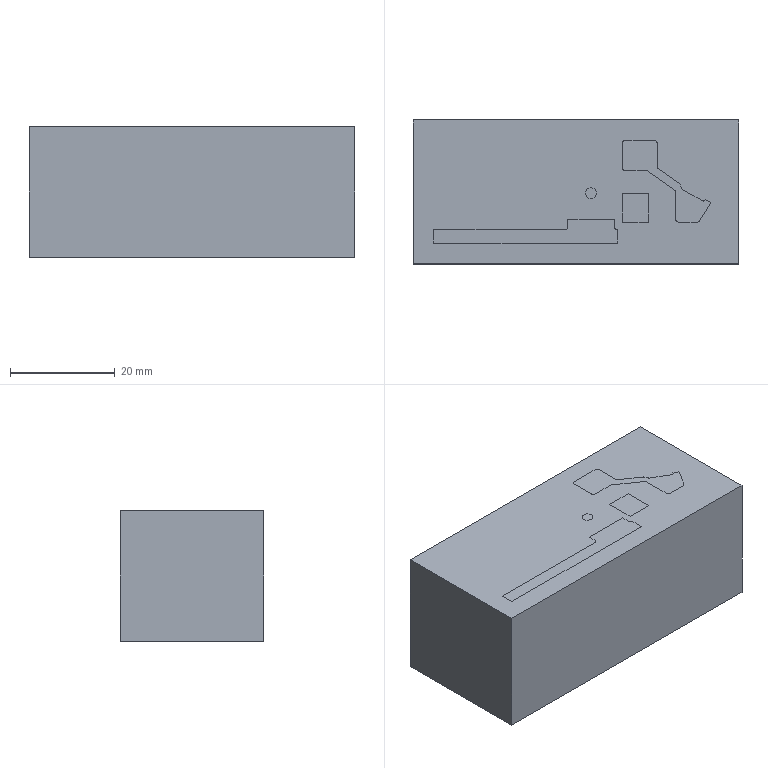Part | NX | features BREP 2 | 2 solids | 75 faces | box 62.287 x 27.499 x 25 mm | volume 78111 mm3 | plane 52 | cylinder 23 | commonest cylinder face diameters 0.9 x7 1.1 x6 3.1 x6 2.1 x1 4.1 x1 72.596 x1